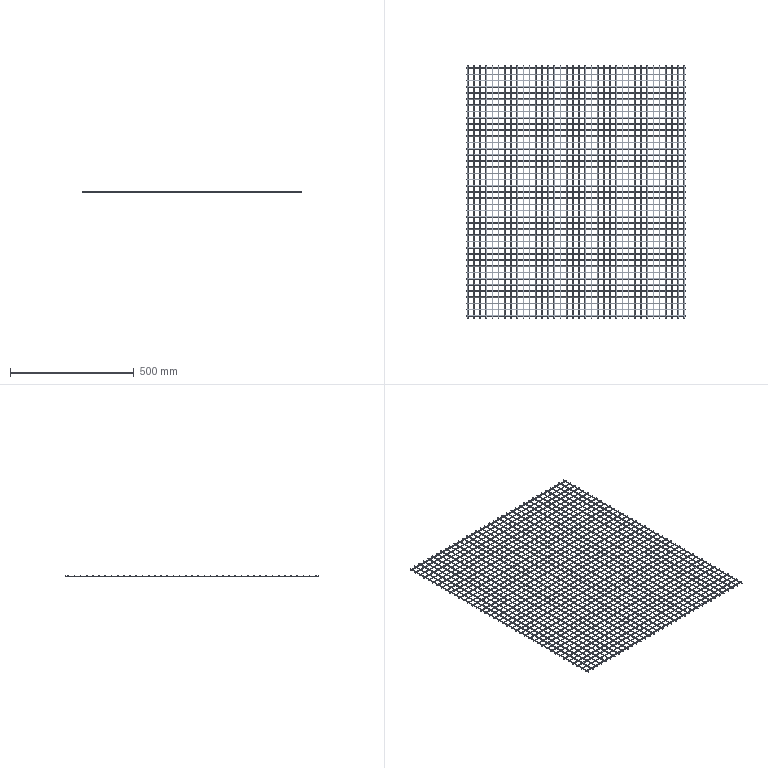Part | STEP file | 750078188 | 77 solids | 308 faces | box 887 x 1018 x 3 mm | volume 516113 mm3 | cylinder 154 | plane 154 | commonest cylinder face diameters 3 x154